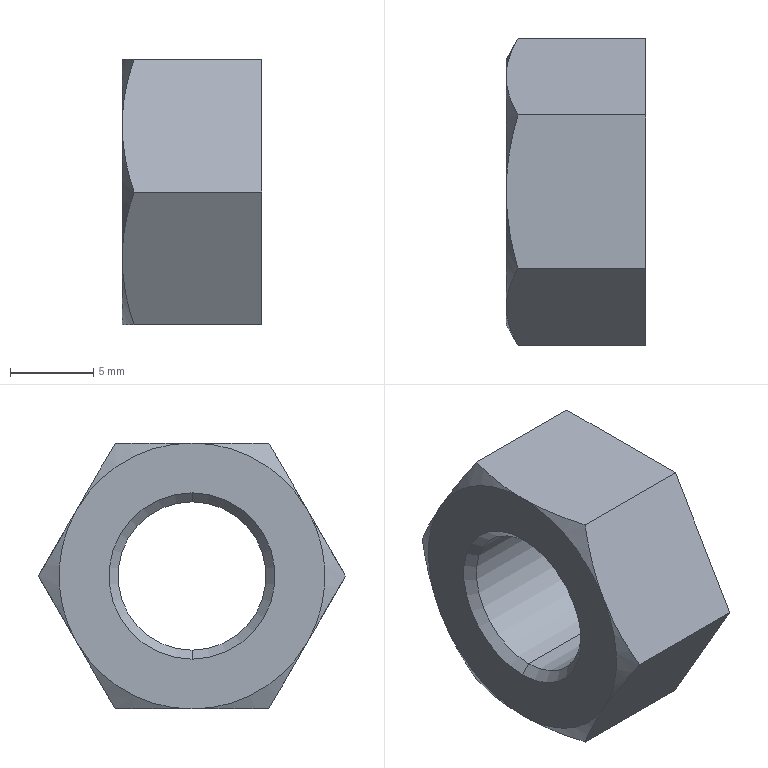Part | SolidWorks | features BaseBody 1 | 1 solid | 20 faces | box 8.4 x 18.475 x 16 mm | volume 1325 mm3 | cone 10 | plane 8 | cylinder 2 | commonest cylinder face diameters 8.917 x2
STEP:
#1=CARTESIAN_POINT('',(7.859,0.,-4.458));
#2=VERTEX_POINT('',#1);
#3=CARTESIAN_POINT('',(7.859,0.,4.458));
#4=VERTEX_POINT('',#3);
#5=CARTESIAN_POINT('',(7.859,0.,0.));
#6=DIRECTION('',(-1.,0.,0.));
#7=DIRECTION('',(0.,0.,1.));
#8=AXIS2_PLACEMENT_3D('',#5,#6,#7);
#9=CIRCLE('',#8,4.458);
#10=EDGE_CURVE('',#2,#4,#9,.T.);
#11=ORIENTED_EDGE('',*,*,#10,.F.);
#12=CARTESIAN_POINT('',(0.5415,0.,-4.458));
#13=VERTEX_POINT('',#12);
#14=CARTESIAN_POINT('',(50.,0.,-4.458));
#15=DIRECTION('',(-1.,0.,0.));
#16=VECTOR('',#15,1000.);
#17=LINE('',#14,#16);
#18=EDGE_CURVE('',#2,#13,#17,.T.);
#19=ORIENTED_EDGE('',*,*,#18,.T.);
#20=CARTESIAN_POINT('',(0.5415,0.,4.458));
#21=VERTEX_POINT('',#20);
#22=CARTESIAN_POINT('',(0.5415,0.,0.));
#23=DIRECTION('',(1.,0.,0.));
#24=DIRECTION('',(0.,0.,1.));
#25=AXIS2_PLACEMENT_3D('',#22,#23,#24);
#26=CIRCLE('',#25,4.458);
#27=EDGE_CURVE('',#21,#13,#26,.T.);
#28=ORIENTED_EDGE('',*,*,#27,.F.);
#29=CARTESIAN_POINT('',(50.,0.,4.458));
#30=DIRECTION('',(-1.,0.,0.));
#31=VECTOR('',#30,1000.);
#32=LINE('',#29,#31);
#33=EDGE_CURVE('',#4,#21,#32,.T.);
#34=ORIENTED_EDGE('',*,*,#33,.F.);
#35=EDGE_LOOP('',(#11,#19,#28,#34));
#36=FACE_OUTER_BOUND('',#35,.T.);
#37=CARTESIAN_POINT('',(50.,0.,0.));
#38=DIRECTION('',(-1.,0.,0.));
#39=DIRECTION('',(0.,0.,1.));
#40=AXIS2_PLACEMENT_3D('',#37,#38,#39);
#41=CYLINDRICAL_SURFACE('',#40,4.458);
#42=ADVANCED_FACE('',(#36),#41,.F.);
#43=ORIENTED_EDGE('',*,*,#27,.T.);
#44=CARTESIAN_POINT('',(0.,0.,-5.));
#45=VERTEX_POINT('',#44);
#46=CARTESIAN_POINT('',(0.,0.,-5.));
#47=DIRECTION('',(-0.7071,0.,-0.7071));
#48=VECTOR('',#47,1000.);
#49=LINE('',#46,#48);
#50=EDGE_CURVE('',#13,#45,#49,.T.);
#51=ORIENTED_EDGE('',*,*,#50,.T.);
#52=CARTESIAN_POINT('',(0.,0.,5.));
#53=VERTEX_POINT('',#52);
#54=CARTESIAN_POINT('',(0.,0.,0.));
#55=DIRECTION('',(1.,0.,0.));
#56=DIRECTION('',(0.,0.,1.));
#57=AXIS2_PLACEMENT_3D('',#54,#55,#56);
#58=CIRCLE('',#57,5.);
#59=EDGE_CURVE('',#53,#45,#58,.T.);
#60=ORIENTED_EDGE('',*,*,#59,.F.);
#61=CARTESIAN_POINT('',(0.,0.,5.));
#62=DIRECTION('',(-0.7071,0.,0.7071));
#63=VECTOR('',#62,1000.);
#64=LINE('',#61,#63);
#65=EDGE_CURVE('',#21,#53,#64,.T.);
#66=ORIENTED_EDGE('',*,*,#65,.F.);
#67=EDGE_LOOP('',(#43,#51,#60,#66));
#68=FACE_OUTER_BOUND('',#67,.T.);
#69=CARTESIAN_POINT('',(0.,0.,0.));
#70=DIRECTION('',(-1.,0.,0.));
#71=DIRECTION('',(0.,0.,1.));
#72=AXIS2_PLACEMENT_3D('',#69,#70,#71);
#73=CONICAL_SURFACE('',#72,5.,0.7854);
#74=ADVANCED_FACE('',(#68),#73,.F.);
#75=ORIENTED_EDGE('',*,*,#10,.T.);
#76=CARTESIAN_POINT('',(8.4,0.,5.));
#77=VERTEX_POINT('',#76);
#78=CARTESIAN_POINT('',(8.4,0.,5.));
#79=DIRECTION('',(0.7071,0.,0.7071));
#80=VECTOR('',#79,1000.);
#81=LINE('',#78,#80);
#82=EDGE_CURVE('',#4,#77,#81,.T.);
#83=ORIENTED_EDGE('',*,*,#82,.T.);
#84=CARTESIAN_POINT('',(8.4,0.,-5.));
#85=VERTEX_POINT('',#84);
#86=CARTESIAN_POINT('',(8.4,0.,0.));
#87=DIRECTION('',(-1.,0.,0.));
#88=DIRECTION('',(0.,0.,-1.));
#89=AXIS2_PLACEMENT_3D('',#86,#87,#88);
#90=CIRCLE('',#89,5.);
#91=EDGE_CURVE('',#85,#77,#90,.T.);
#92=ORIENTED_EDGE('',*,*,#91,.F.);
#93=CARTESIAN_POINT('',(8.4,0.,-5.));
#94=DIRECTION('',(0.7071,0.,-0.7071));
#95=VECTOR('',#94,1000.);
#96=LINE('',#93,#95);
#97=EDGE_CURVE('',#2,#85,#96,.T.);
#98=ORIENTED_EDGE('',*,*,#97,.F.);
#99=EDGE_LOOP('',(#75,#83,#92,#98));
#100=FACE_OUTER_BOUND('',#99,.T.);
#101=CARTESIAN_POINT('',(8.4,0.,0.));
#102=DIRECTION('',(1.,0.,0.));
#103=DIRECTION('',(0.,0.,-1.));
#104=AXIS2_PLACEMENT_3D('',#101,#102,#103);
#105=CONICAL_SURFACE('',#104,5.,0.7854);
#106=ADVANCED_FACE('',(#100),#105,.F.);
#107=ORIENTED_EDGE('',*,*,#18,.F.);
#108=CARTESIAN_POINT('',(7.859,0.,0.));
#109=DIRECTION('',(-1.,0.,0.));
#110=DIRECTION('',(0.,0.,1.));
#111=AXIS2_PLACEMENT_3D('',#108,#109,#110);
#112=CIRCLE('',#111,4.458);
#113=EDGE_CURVE('',#4,#2,#112,.T.);
#114=ORIENTED_EDGE('',*,*,#113,.F.);
#115=ORIENTED_EDGE('',*,*,#33,.T.);
#116=CARTESIAN_POINT('',(0.5415,0.,0.));
#117=DIRECTION('',(1.,0.,0.));
#118=DIRECTION('',(0.,0.,1.));
#119=AXIS2_PLACEMENT_3D('',#116,#117,#118);
#120=CIRCLE('',#119,4.458);
#121=EDGE_CURVE('',#13,#21,#120,.T.);
#122=ORIENTED_EDGE('',*,*,#121,.F.);
#123=EDGE_LOOP('',(#107,#114,#115,#122));
#124=FACE_OUTER_BOUND('',#123,.T.);
#125=CARTESIAN_POINT('',(50.,0.,0.));
#126=DIRECTION('',(-1.,0.,0.));
#127=DIRECTION('',(0.,0.,1.));
#128=AXIS2_PLACEMENT_3D('',#125,#126,#127);
#129=CYLINDRICAL_SURFACE('',#128,4.458);
#130=ADVANCED_FACE('',(#124),#129,.F.);
#131=ORIENTED_EDGE('',*,*,#50,.F.);
#132=ORIENTED_EDGE('',*,*,#121,.T.);
#133=ORIENTED_EDGE('',*,*,#65,.T.);
#134=CARTESIAN_POINT('',(0.,0.,0.));
#135=DIRECTION('',(1.,0.,0.));
#136=DIRECTION('',(0.,0.,1.));
#137=AXIS2_PLACEMENT_3D('',#134,#135,#136);
#138=CIRCLE('',#137,5.);
#139=EDGE_CURVE('',#45,#53,#138,.T.);
#140=ORIENTED_EDGE('',*,*,#139,.F.);
#141=EDGE_LOOP('',(#131,#132,#133,#140));
#142=FACE_OUTER_BOUND('',#141,.T.);
#143=CARTESIAN_POINT('',(0.,0.,0.));
#144=DIRECTION('',(-1.,0.,0.));
#145=DIRECTION('',(0.,0.,1.));
#146=AXIS2_PLACEMENT_3D('',#143,#144,#145);
#147=CONICAL_SURFACE('',#146,5.,0.7854);
#148=ADVANCED_FACE('',(#142),#147,.F.);
#149=ORIENTED_EDGE('',*,*,#82,.F.);
#150=ORIENTED_EDGE('',*,*,#113,.T.);
#151=ORIENTED_EDGE('',*,*,#97,.T.);
#152=CARTESIAN_POINT('',(8.4,0.,0.));
#153=DIRECTION('',(-1.,0.,0.));
#154=DIRECTION('',(0.,0.,-1.));
#155=AXIS2_PLACEMENT_3D('',#152,#153,#154);
#156=CIRCLE('',#155,5.);
#157=EDGE_CURVE('',#77,#85,#156,.T.);
#158=ORIENTED_EDGE('',*,*,#157,.F.);
#159=EDGE_LOOP('',(#149,#150,#151,#158));
#160=FACE_OUTER_BOUND('',#159,.T.);
#161=CARTESIAN_POINT('',(8.4,0.,0.));
#162=DIRECTION('',(1.,0.,0.));
#163=DIRECTION('',(0.,0.,-1.));
#164=AXIS2_PLACEMENT_3D('',#161,#162,#163);
#165=CONICAL_SURFACE('',#164,5.,0.7854);
#166=ADVANCED_FACE('',(#160),#165,.F.);
#167=CARTESIAN_POINT('',(0.,-6.928,4.));
#168=VERTEX_POINT('',#167);
#169=CARTESIAN_POINT('',(0.,0.,8.));
#170=VERTEX_POINT('',#169);
#171=CARTESIAN_POINT('',(0.,0.,0.));
#172=DIRECTION('',(-1.,0.,0.));
#173=DIRECTION('',(0.,0.,-1.));
#174=AXIS2_PLACEMENT_3D('',#171,#172,#173);
#175=CIRCLE('',#174,8.);
#176=EDGE_CURVE('',#168,#170,#175,.T.);
#177=ORIENTED_EDGE('',*,*,#176,.T.);
#178=CARTESIAN_POINT('',(0.,6.928,4.));
#179=VERTEX_POINT('',#178);
#180=CARTESIAN_POINT('',(0.,0.,0.));
#181=DIRECTION('',(-1.,0.,0.));
#182=DIRECTION('',(0.,0.,-1.));
#183=AXIS2_PLACEMENT_3D('',#180,#181,#182);
#184=CIRCLE('',#183,8.);
#185=EDGE_CURVE('',#170,#179,#184,.T.);
#186=ORIENTED_EDGE('',*,*,#185,.T.);
#187=CARTESIAN_POINT('',(0.,6.928,-4.));
#188=VERTEX_POINT('',#187);
#189=CARTESIAN_POINT('',(0.,0.,0.));
#190=DIRECTION('',(-1.,0.,0.));
#191=DIRECTION('',(0.,0.,-1.));
#192=AXIS2_PLACEMENT_3D('',#189,#190,#191);
#193=CIRCLE('',#192,8.);
#194=EDGE_CURVE('',#179,#188,#193,.T.);
#195=ORIENTED_EDGE('',*,*,#194,.T.);
#196=CARTESIAN_POINT('',(0.,0.,-8.));
#197=VERTEX_POINT('',#196);
#198=CARTESIAN_POINT('',(0.,0.,0.));
#199=DIRECTION('',(-1.,0.,0.));
#200=DIRECTION('',(0.,0.,-1.));
#201=AXIS2_PLACEMENT_3D('',#198,#199,#200);
#202=CIRCLE('',#201,8.);
#203=EDGE_CURVE('',#188,#197,#202,.T.);
#204=ORIENTED_EDGE('',*,*,#203,.T.);
#205=CARTESIAN_POINT('',(0.,-6.928,-4.));
#206=VERTEX_POINT('',#205);
#207=CARTESIAN_POINT('',(0.,0.,0.));
#208=DIRECTION('',(-1.,0.,0.));
#209=DIRECTION('',(0.,0.,-1.));
#210=AXIS2_PLACEMENT_3D('',#207,#208,#209);
#211=CIRCLE('',#210,8.);
#212=EDGE_CURVE('',#197,#206,#211,.T.);
#213=ORIENTED_EDGE('',*,*,#212,.T.);
#214=CARTESIAN_POINT('',(0.,0.,0.));
#215=DIRECTION('',(-1.,0.,0.));
#216=DIRECTION('',(0.,0.,-1.));
#217=AXIS2_PLACEMENT_3D('',#214,#215,#216);
#218=CIRCLE('',#217,8.);
#219=EDGE_CURVE('',#206,#168,#218,.T.);
#220=ORIENTED_EDGE('',*,*,#219,.T.);
#221=EDGE_LOOP('',(#177,#186,#195,#204,#213,#220));
#222=FACE_OUTER_BOUND('',#221,.T.);
#223=ORIENTED_EDGE('',*,*,#59,.T.);
#224=ORIENTED_EDGE('',*,*,#139,.T.);
#225=EDGE_LOOP('',(#223,#224));
#226=FACE_BOUND('',#225,.T.);
#227=CARTESIAN_POINT('',(0.,8.,0.));
#228=DIRECTION('',(-1.,0.,0.));
#229=DIRECTION('',(0.,0.,1.));
#230=AXIS2_PLACEMENT_3D('',#227,#228,#229);
#231=PLANE('',#230);
#232=ADVANCED_FACE('',(#222,#226),#231,.T.);
#233=ORIENTED_EDGE('',*,*,#91,.T.);
#234=ORIENTED_EDGE('',*,*,#157,.T.);
#235=EDGE_LOOP('',(#233,#234));
#236=FACE_BOUND('',#235,.T.);
#237=CARTESIAN_POINT('',(8.4,-9.238,0.));
#238=VERTEX_POINT('',#237);
#239=CARTESIAN_POINT('',(8.4,-4.619,-8.));
#240=VERTEX_POINT('',#239);
#241=CARTESIAN_POINT('',(8.4,-9.238,0.));
#242=DIRECTION('',(0.,0.5,-0.866));
#243=VECTOR('',#242,1000.);
#244=LINE('',#241,#243);
#245=EDGE_CURVE('',#238,#240,#244,.T.);
#246=ORIENTED_EDGE('',*,*,#245,.T.);
#247=CARTESIAN_POINT('',(8.4,4.619,-8.));
#248=VERTEX_POINT('',#247);
#249=CARTESIAN_POINT('',(8.4,5.,-8.));
#250=DIRECTION('',(0.,1.,0.));
#251=VECTOR('',#250,1000.);
#252=LINE('',#249,#251);
#253=EDGE_CURVE('',#240,#248,#252,.T.);
#254=ORIENTED_EDGE('',*,*,#253,.T.);
#255=CARTESIAN_POINT('',(8.4,9.238,0.));
#256=VERTEX_POINT('',#255);
#257=CARTESIAN_POINT('',(8.4,4.619,-8.));
#258=DIRECTION('',(0.,0.5,0.866));
#259=VECTOR('',#258,1000.);
#260=LINE('',#257,#259);
#261=EDGE_CURVE('',#248,#256,#260,.T.);
#262=ORIENTED_EDGE('',*,*,#261,.T.);
#263=CARTESIAN_POINT('',(8.4,4.619,8.));
#264=VERTEX_POINT('',#263);
#265=CARTESIAN_POINT('',(8.4,9.238,0.));
#266=DIRECTION('',(0.,-0.5,0.866));
#267=VECTOR('',#266,1000.);
#268=LINE('',#265,#267);
#269=EDGE_CURVE('',#256,#264,#268,.T.);
#270=ORIENTED_EDGE('',*,*,#269,.T.);
#271=CARTESIAN_POINT('',(8.4,-4.619,8.));
#272=VERTEX_POINT('',#271);
#273=CARTESIAN_POINT('',(8.4,5.,8.));
#274=DIRECTION('',(0.,-1.,0.));
#275=VECTOR('',#274,1000.);
#276=LINE('',#273,#275);
#277=EDGE_CURVE('',#264,#272,#276,.T.);
#278=ORIENTED_EDGE('',*,*,#277,.T.);
#279=CARTESIAN_POINT('',(8.4,-4.619,8.));
#280=DIRECTION('',(0.,-0.5,-0.866));
#281=VECTOR('',#280,1000.);
#282=LINE('',#279,#281);
#283=EDGE_CURVE('',#272,#238,#282,.T.);
#284=ORIENTED_EDGE('',*,*,#283,.T.);
#285=EDGE_LOOP('',(#246,#254,#262,#270,#278,#284));
#286=FACE_OUTER_BOUND('',#285,.T.);
#287=CARTESIAN_POINT('',(8.4,5.,0.));
#288=DIRECTION('',(1.,0.,0.));
#289=DIRECTION('',(0.,0.,-1.));
#290=AXIS2_PLACEMENT_3D('',#287,#288,#289);
#291=PLANE('',#290);
#292=ADVANCED_FACE('',(#236,#286),#291,.T.);
#293=ORIENTED_EDGE('',*,*,#185,.F.);
#294=CARTESIAN_POINT('',(0.7145,4.619,8.));
#295=VERTEX_POINT('',#294);
#296=CARTESIAN_POINT('',(0.,0.,8.));
#297=CARTESIAN_POINT('',(0.,0.7882,8.));
#298=CARTESIAN_POINT('',(0.06831,1.566,8.));
#299=CARTESIAN_POINT('',(0.3171,3.104,8.));
#300=CARTESIAN_POINT('',(0.4967,3.864,8.));
#301=CARTESIAN_POINT('',(0.7145,4.619,8.));
#302=B_SPLINE_CURVE_WITH_KNOTS('',3,(#296,#297,#298,#299,#300,#301),.UNSPECIFIED.,.F.,.F.,(4,2,4),(0.,0.002337,0.004674),.UNSPECIFIED.);
#303=EDGE_CURVE('',#170,#295,#302,.T.);
#304=ORIENTED_EDGE('',*,*,#303,.T.);
#305=CARTESIAN_POINT('',(0.7145,4.619,8.));
#306=CARTESIAN_POINT('',(0.4967,4.996,7.347));
#307=CARTESIAN_POINT('',(0.3171,5.376,6.688));
#308=CARTESIAN_POINT('',(0.06831,6.145,5.356));
#309=CARTESIAN_POINT('',(0.,6.534,4.683));
#310=CARTESIAN_POINT('',(0.,6.928,4.));
#311=B_SPLINE_CURVE_WITH_KNOTS('',3,(#305,#306,#307,#308,#309,#310),.UNSPECIFIED.,.F.,.F.,(4,2,4),(0.,0.002337,0.004674),.UNSPECIFIED.);
#312=EDGE_CURVE('',#295,#179,#311,.T.);
#313=ORIENTED_EDGE('',*,*,#312,.T.);
#314=EDGE_LOOP('',(#293,#304,#313));
#315=FACE_OUTER_BOUND('',#314,.T.);
#316=CARTESIAN_POINT('',(0.7188,0.,0.));
#317=DIRECTION('',(1.,0.,0.));
#318=DIRECTION('',(0.,0.,-1.));
#319=AXIS2_PLACEMENT_3D('',#316,#317,#318);
#320=CONICAL_SURFACE('',#319,9.245,1.047);
#321=ADVANCED_FACE('',(#315),#320,.T.);
#322=ORIENTED_EDGE('',*,*,#176,.F.);
#323=CARTESIAN_POINT('',(0.7145,-4.619,8.));
#324=VERTEX_POINT('',#323);
#325=CARTESIAN_POINT('',(0.,-6.928,4.));
#326=CARTESIAN_POINT('',(0.,-6.534,4.683));
#327=CARTESIAN_POINT('',(0.06831,-6.145,5.356));
#328=CARTESIAN_POINT('',(0.3171,-5.376,6.688));
#329=CARTESIAN_POINT('',(0.4967,-4.996,7.347));
#330=CARTESIAN_POINT('',(0.7145,-4.619,8.));
#331=B_SPLINE_CURVE_WITH_KNOTS('',3,(#325,#326,#327,#328,#329,#330),.UNSPECIFIED.,.F.,.F.,(4,2,4),(0.,0.002337,0.004674),.UNSPECIFIED.);
#332=EDGE_CURVE('',#168,#324,#331,.T.);
#333=ORIENTED_EDGE('',*,*,#332,.T.);
#334=CARTESIAN_POINT('',(0.7145,-4.619,8.));
#335=CARTESIAN_POINT('',(0.4967,-3.864,8.));
#336=CARTESIAN_POINT('',(0.3171,-3.104,8.));
#337=CARTESIAN_POINT('',(0.06831,-1.566,8.));
#338=CARTESIAN_POINT('',(0.,-0.7882,8.));
#339=CARTESIAN_POINT('',(0.,0.,8.));
#340=B_SPLINE_CURVE_WITH_KNOTS('',3,(#334,#335,#336,#337,#338,#339),.UNSPECIFIED.,.F.,.F.,(4,2,4),(0.,0.002337,0.004674),.UNSPECIFIED.);
#341=EDGE_CURVE('',#324,#170,#340,.T.);
#342=ORIENTED_EDGE('',*,*,#341,.T.);
#343=EDGE_LOOP('',(#322,#333,#342));
#344=FACE_OUTER_BOUND('',#343,.T.);
#345=CARTESIAN_POINT('',(0.7188,0.,0.));
#346=DIRECTION('',(1.,0.,0.));
#347=DIRECTION('',(0.,0.,-1.));
#348=AXIS2_PLACEMENT_3D('',#345,#346,#347);
#349=CONICAL_SURFACE('',#348,9.245,1.047);
#350=ADVANCED_FACE('',(#344),#349,.T.);
#351=CARTESIAN_POINT('',(0.7145,-9.238,-0.000000043));
#352=VERTEX_POINT('',#351);
#353=CARTESIAN_POINT('',(0.7145,-9.238,-0.000000043));
#354=CARTESIAN_POINT('',(0.4967,-8.86,0.6534));
#355=CARTESIAN_POINT('',(0.3171,-8.48,1.312));
#356=CARTESIAN_POINT('',(0.06831,-7.711,2.644));
#357=CARTESIAN_POINT('',(0.,-7.322,3.317));
#358=CARTESIAN_POINT('',(0.,-6.928,4.));
#359=B_SPLINE_CURVE_WITH_KNOTS('',3,(#353,#354,#355,#356,#357,#358),.UNSPECIFIED.,.F.,.F.,(4,2,4),(0.,0.002337,0.004674),.UNSPECIFIED.);
#360=EDGE_CURVE('',#352,#168,#359,.T.);
#361=ORIENTED_EDGE('',*,*,#360,.T.);
#362=ORIENTED_EDGE('',*,*,#219,.F.);
#363=CARTESIAN_POINT('',(0.,-6.928,-4.));
#364=CARTESIAN_POINT('',(0.,-7.322,-3.317));
#365=CARTESIAN_POINT('',(0.06831,-7.711,-2.644));
#366=CARTESIAN_POINT('',(0.3171,-8.48,-1.312));
#367=CARTESIAN_POINT('',(0.4967,-8.86,-0.6534));
#368=CARTESIAN_POINT('',(0.7145,-9.238,-0.000000043));
#369=B_SPLINE_CURVE_WITH_KNOTS('',3,(#363,#364,#365,#366,#367,#368),.UNSPECIFIED.,.F.,.F.,(4,2,4),(0.,0.002337,0.004674),.UNSPECIFIED.);
#370=EDGE_CURVE('',#206,#352,#369,.T.);
#371=ORIENTED_EDGE('',*,*,#370,.T.);
#372=EDGE_LOOP('',(#361,#362,#371));
#373=FACE_OUTER_BOUND('',#372,.T.);
#374=CARTESIAN_POINT('',(0.7188,0.,0.));
#375=DIRECTION('',(1.,0.,0.));
#376=DIRECTION('',(0.,0.,-1.));
#377=AXIS2_PLACEMENT_3D('',#374,#375,#376);
#378=CONICAL_SURFACE('',#377,9.245,1.047);
#379=ADVANCED_FACE('',(#373),#378,.T.);
#380=CARTESIAN_POINT('',(0.7145,-4.619,-8.));
#381=VERTEX_POINT('',#380);
#382=CARTESIAN_POINT('',(0.7145,-4.619,-8.));
#383=CARTESIAN_POINT('',(0.4967,-4.996,-7.347));
#384=CARTESIAN_POINT('',(0.3171,-5.376,-6.688));
#385=CARTESIAN_POINT('',(0.06831,-6.145,-5.356));
#386=CARTESIAN_POINT('',(0.,-6.534,-4.683));
#387=CARTESIAN_POINT('',(0.,-6.928,-4.));
#388=B_SPLINE_CURVE_WITH_KNOTS('',3,(#382,#383,#384,#385,#386,#387),.UNSPECIFIED.,.F.,.F.,(4,2,4),(0.,0.002337,0.004674),.UNSPECIFIED.);
#389=EDGE_CURVE('',#381,#206,#388,.T.);
#390=ORIENTED_EDGE('',*,*,#389,.T.);
#391=ORIENTED_EDGE('',*,*,#212,.F.);
#392=CARTESIAN_POINT('',(0.,0.,-8.));
#393=CARTESIAN_POINT('',(0.,-0.7882,-8.));
#394=CARTESIAN_POINT('',(0.06831,-1.566,-8.));
#395=CARTESIAN_POINT('',(0.3171,-3.104,-8.));
#396=CARTESIAN_POINT('',(0.4967,-3.864,-8.));
#397=CARTESIAN_POINT('',(0.7145,-4.619,-8.));
#398=B_SPLINE_CURVE_WITH_KNOTS('',3,(#392,#393,#394,#395,#396,#397),.UNSPECIFIED.,.F.,.F.,(4,2,4),(0.,0.002337,0.004674),.UNSPECIFIED.);
#399=EDGE_CURVE('',#197,#381,#398,.T.);
#400=ORIENTED_EDGE('',*,*,#399,.T.);
#401=EDGE_LOOP('',(#390,#391,#400));
#402=FACE_OUTER_BOUND('',#401,.T.);
#403=CARTESIAN_POINT('',(0.7188,0.,0.));
#404=DIRECTION('',(1.,0.,0.));
#405=DIRECTION('',(0.,0.,-1.));
#406=AXIS2_PLACEMENT_3D('',#403,#404,#405);
#407=CONICAL_SURFACE('',#406,9.245,1.047);
#408=ADVANCED_FACE('',(#402),#407,.T.);
#409=CARTESIAN_POINT('',(0.7145,4.619,-8.));
#410=VERTEX_POINT('',#409);
#411=CARTESIAN_POINT('',(0.7145,4.619,-8.));
#412=CARTESIAN_POINT('',(0.4967,3.864,-8.));
#413=CARTESIAN_POINT('',(0.3171,3.104,-8.));
#414=CARTESIAN_POINT('',(0.06831,1.566,-8.));
#415=CARTESIAN_POINT('',(0.,0.7882,-8.));
#416=CARTESIAN_POINT('',(0.,0.,-8.));
#417=B_SPLINE_CURVE_WITH_KNOTS('',3,(#411,#412,#413,#414,#415,#416),.UNSPECIFIED.,.F.,.F.,(4,2,4),(0.,0.002337,0.004674),.UNSPECIFIED.);
#418=EDGE_CURVE('',#410,#197,#417,.T.);
#419=ORIENTED_EDGE('',*,*,#418,.T.);
#420=ORIENTED_EDGE('',*,*,#203,.F.);
#421=CARTESIAN_POINT('',(0.,6.928,-4.));
#422=CARTESIAN_POINT('',(0.,6.534,-4.683));
#423=CARTESIAN_POINT('',(0.06831,6.145,-5.356));
#424=CARTESIAN_POINT('',(0.3171,5.376,-6.688));
#425=CARTESIAN_POINT('',(0.4967,4.996,-7.347));
#426=CARTESIAN_POINT('',(0.7145,4.619,-8.));
#427=B_SPLINE_CURVE_WITH_KNOTS('',3,(#421,#422,#423,#424,#425,#426),.UNSPECIFIED.,.F.,.F.,(4,2,4),(0.,0.002337,0.004674),.UNSPECIFIED.);
#428=EDGE_CURVE('',#188,#410,#427,.T.);
#429=ORIENTED_EDGE('',*,*,#428,.T.);
#430=EDGE_LOOP('',(#419,#420,#429));
#431=FACE_OUTER_BOUND('',#430,.T.);
#432=CARTESIAN_POINT('',(0.7188,0.,0.));
#433=DIRECTION('',(1.,0.,0.));
#434=DIRECTION('',(0.,0.,-1.));
#435=AXIS2_PLACEMENT_3D('',#432,#433,#434);
#436=CONICAL_SURFACE('',#435,9.245,1.047);
#437=ADVANCED_FACE('',(#431),#436,.T.);
#438=CARTESIAN_POINT('',(0.7145,9.238,0.000000043));
#439=VERTEX_POINT('',#438);
#440=CARTESIAN_POINT('',(0.7145,9.238,0.000000043));
#441=CARTESIAN_POINT('',(0.4967,8.86,-0.6534));
#442=CARTESIAN_POINT('',(0.3171,8.48,-1.312));
#443=CARTESIAN_POINT('',(0.06831,7.711,-2.644));
#444=CARTESIAN_POINT('',(0.,7.322,-3.317));
#445=CARTESIAN_POINT('',(0.,6.928,-4.));
#446=B_SPLINE_CURVE_WITH_KNOTS('',3,(#440,#441,#442,#443,#444,#445),.UNSPECIFIED.,.F.,.F.,(4,2,4),(0.,0.002337,0.004674),.UNSPECIFIED.);
#447=EDGE_CURVE('',#439,#188,#446,.T.);
#448=ORIENTED_EDGE('',*,*,#447,.T.);
#449=ORIENTED_EDGE('',*,*,#194,.F.);
#450=CARTESIAN_POINT('',(0.,6.928,4.));
#451=CARTESIAN_POINT('',(0.,7.322,3.317));
#452=CARTESIAN_POINT('',(0.06831,7.711,2.644));
#453=CARTESIAN_POINT('',(0.3171,8.48,1.312));
#454=CARTESIAN_POINT('',(0.4967,8.86,0.6534));
#455=CARTESIAN_POINT('',(0.7145,9.238,0.000000043));
#456=B_SPLINE_CURVE_WITH_KNOTS('',3,(#450,#451,#452,#453,#454,#455),.UNSPECIFIED.,.F.,.F.,(4,2,4),(0.,0.002337,0.004674),.UNSPECIFIED.);
#457=EDGE_CURVE('',#179,#439,#456,.T.);
#458=ORIENTED_EDGE('',*,*,#457,.T.);
#459=EDGE_LOOP('',(#448,#449,#458));
#460=FACE_OUTER_BOUND('',#459,.T.);
#461=CARTESIAN_POINT('',(0.7188,0.,0.));
#462=DIRECTION('',(1.,0.,0.));
#463=DIRECTION('',(0.,0.,-1.));
#464=AXIS2_PLACEMENT_3D('',#461,#462,#463);
#465=CONICAL_SURFACE('',#464,9.245,1.047);
#466=ADVANCED_FACE('',(#460),#465,.T.);
#467=ORIENTED_EDGE('',*,*,#418,.F.);
#468=CARTESIAN_POINT('',(8.4,4.619,-8.));
#469=DIRECTION('',(-1.,0.,0.));
#470=VECTOR('',#469,1000.);
#471=LINE('',#468,#470);
#472=EDGE_CURVE('',#248,#410,#471,.T.);
#473=ORIENTED_EDGE('',*,*,#472,.F.);
#474=ORIENTED_EDGE('',*,*,#253,.F.);
#475=CARTESIAN_POINT('',(8.4,-4.619,-8.));
#476=DIRECTION('',(1.,0.,0.));
#477=VECTOR('',#476,1000.);
#478=LINE('',#475,#477);
#479=EDGE_CURVE('',#381,#240,#478,.T.);
#480=ORIENTED_EDGE('',*,*,#479,.F.);
#481=ORIENTED_EDGE('',*,*,#399,.F.);
#482=EDGE_LOOP('',(#467,#473,#474,#480,#481));
#483=FACE_OUTER_BOUND('',#482,.T.);
#484=CARTESIAN_POINT('',(8.4,-4.619,-8.));
#485=DIRECTION('',(0.,0.,1.));
#486=DIRECTION('',(1.,0.,0.));
#487=AXIS2_PLACEMENT_3D('',#484,#485,#486);
#488=PLANE('',#487);
#489=ADVANCED_FACE('',(#483),#488,.F.);
#490=ORIENTED_EDGE('',*,*,#389,.F.);
#491=ORIENTED_EDGE('',*,*,#479,.T.);
#492=ORIENTED_EDGE('',*,*,#245,.F.);
#493=CARTESIAN_POINT('',(8.4,-9.238,0.));
#494=DIRECTION('',(1.,0.,0.));
#495=VECTOR('',#494,1000.);
#496=LINE('',#493,#495);
#497=EDGE_CURVE('',#352,#238,#496,.T.);
#498=ORIENTED_EDGE('',*,*,#497,.F.);
#499=ORIENTED_EDGE('',*,*,#370,.F.);
#500=EDGE_LOOP('',(#490,#491,#492,#498,#499));
#501=FACE_OUTER_BOUND('',#500,.T.);
#502=CARTESIAN_POINT('',(8.4,-9.238,0.));
#503=DIRECTION('',(0.,0.866,0.5));
#504=DIRECTION('',(0.,-0.5,0.866));
#505=AXIS2_PLACEMENT_3D('',#502,#503,#504);
#506=PLANE('',#505);
#507=ADVANCED_FACE('',(#501),#506,.F.);
#508=ORIENTED_EDGE('',*,*,#360,.F.);
#509=ORIENTED_EDGE('',*,*,#497,.T.);
#510=ORIENTED_EDGE('',*,*,#283,.F.);
#511=CARTESIAN_POINT('',(8.4,-4.619,8.));
#512=DIRECTION('',(1.,0.,0.));
#513=VECTOR('',#512,1000.);
#514=LINE('',#511,#513);
#515=EDGE_CURVE('',#324,#272,#514,.T.);
#516=ORIENTED_EDGE('',*,*,#515,.F.);
#517=ORIENTED_EDGE('',*,*,#332,.F.);
#518=EDGE_LOOP('',(#508,#509,#510,#516,#517));
#519=FACE_OUTER_BOUND('',#518,.T.);
#520=CARTESIAN_POINT('',(8.4,-4.619,8.));
#521=DIRECTION('',(0.,0.866,-0.5));
#522=DIRECTION('',(0.,0.5,0.866));
#523=AXIS2_PLACEMENT_3D('',#520,#521,#522);
#524=PLANE('',#523);
#525=ADVANCED_FACE('',(#519),#524,.F.);
#526=ORIENTED_EDGE('',*,*,#341,.F.);
#527=ORIENTED_EDGE('',*,*,#515,.T.);
#528=ORIENTED_EDGE('',*,*,#277,.F.);
#529=CARTESIAN_POINT('',(8.4,4.619,8.));
#530=DIRECTION('',(1.,0.,0.));
#531=VECTOR('',#530,1000.);
#532=LINE('',#529,#531);
#533=EDGE_CURVE('',#295,#264,#532,.T.);
#534=ORIENTED_EDGE('',*,*,#533,.F.);
#535=ORIENTED_EDGE('',*,*,#303,.F.);
#536=EDGE_LOOP('',(#526,#527,#528,#534,#535));
#537=FACE_OUTER_BOUND('',#536,.T.);
#538=CARTESIAN_POINT('',(8.4,4.619,8.));
#539=DIRECTION('',(0.,0.,-1.));
#540=DIRECTION('',(-1.,0.,0.));
#541=AXIS2_PLACEMENT_3D('',#538,#539,#540);
#542=PLANE('',#541);
#543=ADVANCED_FACE('',(#537),#542,.F.);
#544=ORIENTED_EDGE('',*,*,#312,.F.);
#545=ORIENTED_EDGE('',*,*,#533,.T.);
#546=ORIENTED_EDGE('',*,*,#269,.F.);
#547=CARTESIAN_POINT('',(8.4,9.238,0.));
#548=DIRECTION('',(1.,0.,0.));
#549=VECTOR('',#548,1000.);
#550=LINE('',#547,#549);
#551=EDGE_CURVE('',#439,#256,#550,.T.);
#552=ORIENTED_EDGE('',*,*,#551,.F.);
#553=ORIENTED_EDGE('',*,*,#457,.F.);
#554=EDGE_LOOP('',(#544,#545,#546,#552,#553));
#555=FACE_OUTER_BOUND('',#554,.T.);
#556=CARTESIAN_POINT('',(8.4,9.238,0.));
#557=DIRECTION('',(0.,-0.866,-0.5));
#558=DIRECTION('',(0.,0.5,-0.866));
#559=AXIS2_PLACEMENT_3D('',#556,#557,#558);
#560=PLANE('',#559);
#561=ADVANCED_FACE('',(#555),#560,.F.);
#562=ORIENTED_EDGE('',*,*,#447,.F.);
#563=ORIENTED_EDGE('',*,*,#551,.T.);
#564=ORIENTED_EDGE('',*,*,#261,.F.);
#565=ORIENTED_EDGE('',*,*,#472,.T.);
#566=ORIENTED_EDGE('',*,*,#428,.F.);
#567=EDGE_LOOP('',(#562,#563,#564,#565,#566));
#568=FACE_OUTER_BOUND('',#567,.T.);
#569=CARTESIAN_POINT('',(8.4,4.619,-8.));
#570=DIRECTION('',(0.,-0.866,0.5));
#571=DIRECTION('',(0.,-0.5,-0.866));
#572=AXIS2_PLACEMENT_3D('',#569,#570,#571);
#573=PLANE('',#572);
#574=ADVANCED_FACE('',(#568),#573,.F.);
#575=CLOSED_SHELL('',(#42,#74,#106,#130,#148,#166,#232,#292,#321,#350,#379,#408,#437,#466,#489,#507,#525,#543,#561,#574));
#576=MANIFOLD_SOLID_BREP('',#575);
#577=CARTESIAN_POINT('',(0.,0.,0.));
#578=DIRECTION('',(0.,0.,1.));
#579=DIRECTION('',(1.,0.,0.));
#580=AXIS2_PLACEMENT_3D('',#577,#578,#579);
#581=(LENGTH_UNIT()NAMED_UNIT(*)SI_UNIT(.MILLI.,.METRE.));
#582=UNCERTAINTY_MEASURE_WITH_UNIT(LENGTH_MEASURE(0.00001),#581,'','');
#583=(NAMED_UNIT(*)PLANE_ANGLE_UNIT()SI_UNIT($,.RADIAN.));
#584=(NAMED_UNIT(*)SI_UNIT($,.STERADIAN.)SOLID_ANGLE_UNIT());
#585=(GEOMETRIC_REPRESENTATION_CONTEXT(3)GLOBAL_UNCERTAINTY_ASSIGNED_CONTEXT((#582))GLOBAL_UNIT_ASSIGNED_CONTEXT((#581,#583,#584))REPRESENTATION_CONTEXT('',''));
#586=ADVANCED_BREP_SHAPE_REPRESENTATION('',(#576,#580),#585);